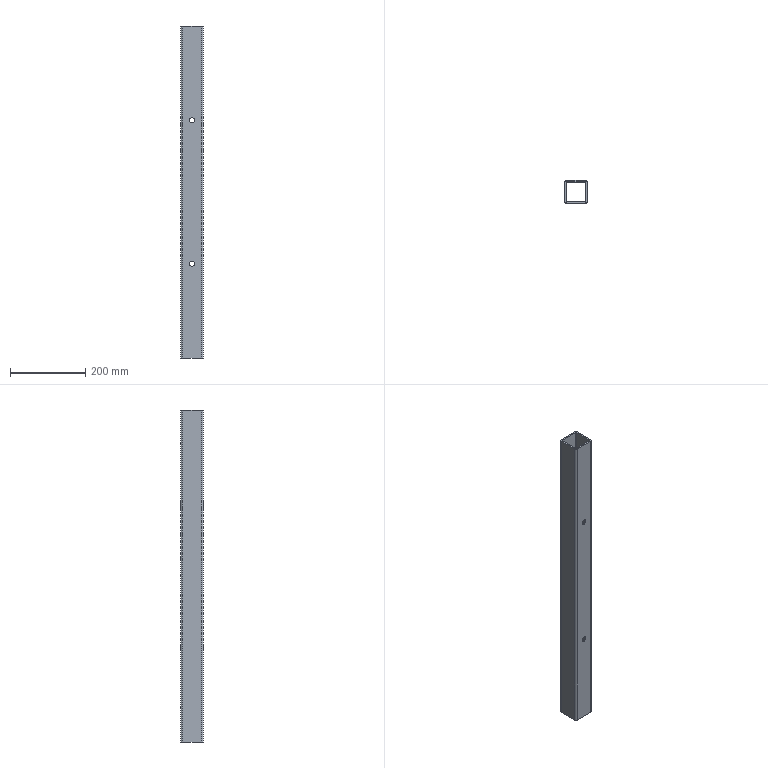Part | STEP file | square steel tube 60x60x4x880 | 1 solid | 36 faces | box 60 x 60 x 880 mm | volume 767950 mm3 | cylinder 26 | plane 10 | commonest cylinder face diameters 4.2 x10 13 x8 2 x4 10 x4